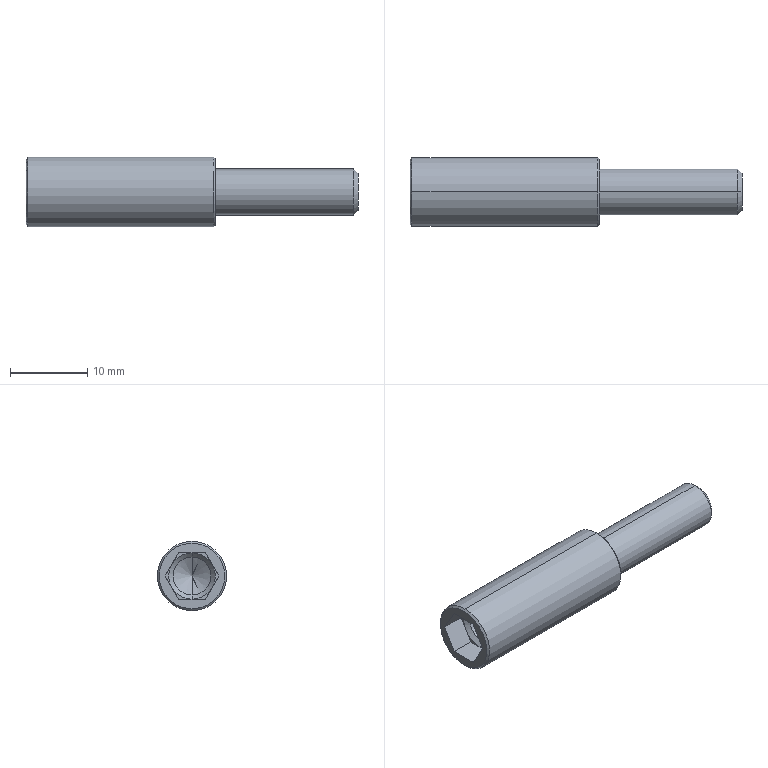Part | STEP file | SI-40X75-S-B1N-2-4 | 1 solid | 31 faces | box 43 x 9 x 9 mm | volume 1649 mm3 | plane 15 | cone 10 | cylinder 6 | commonest cylinder face diameters 4.917 x2 6 x2 9 x2